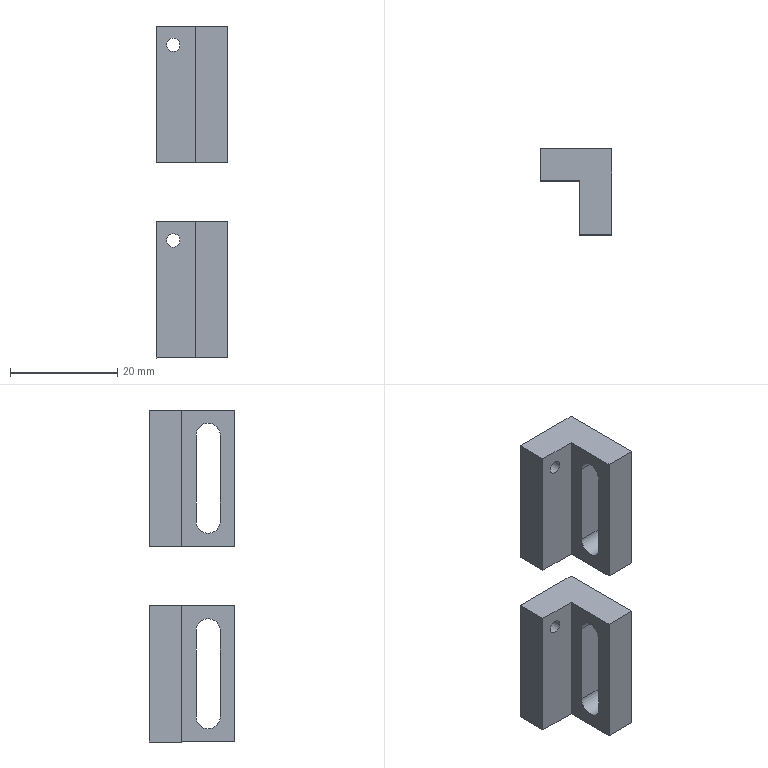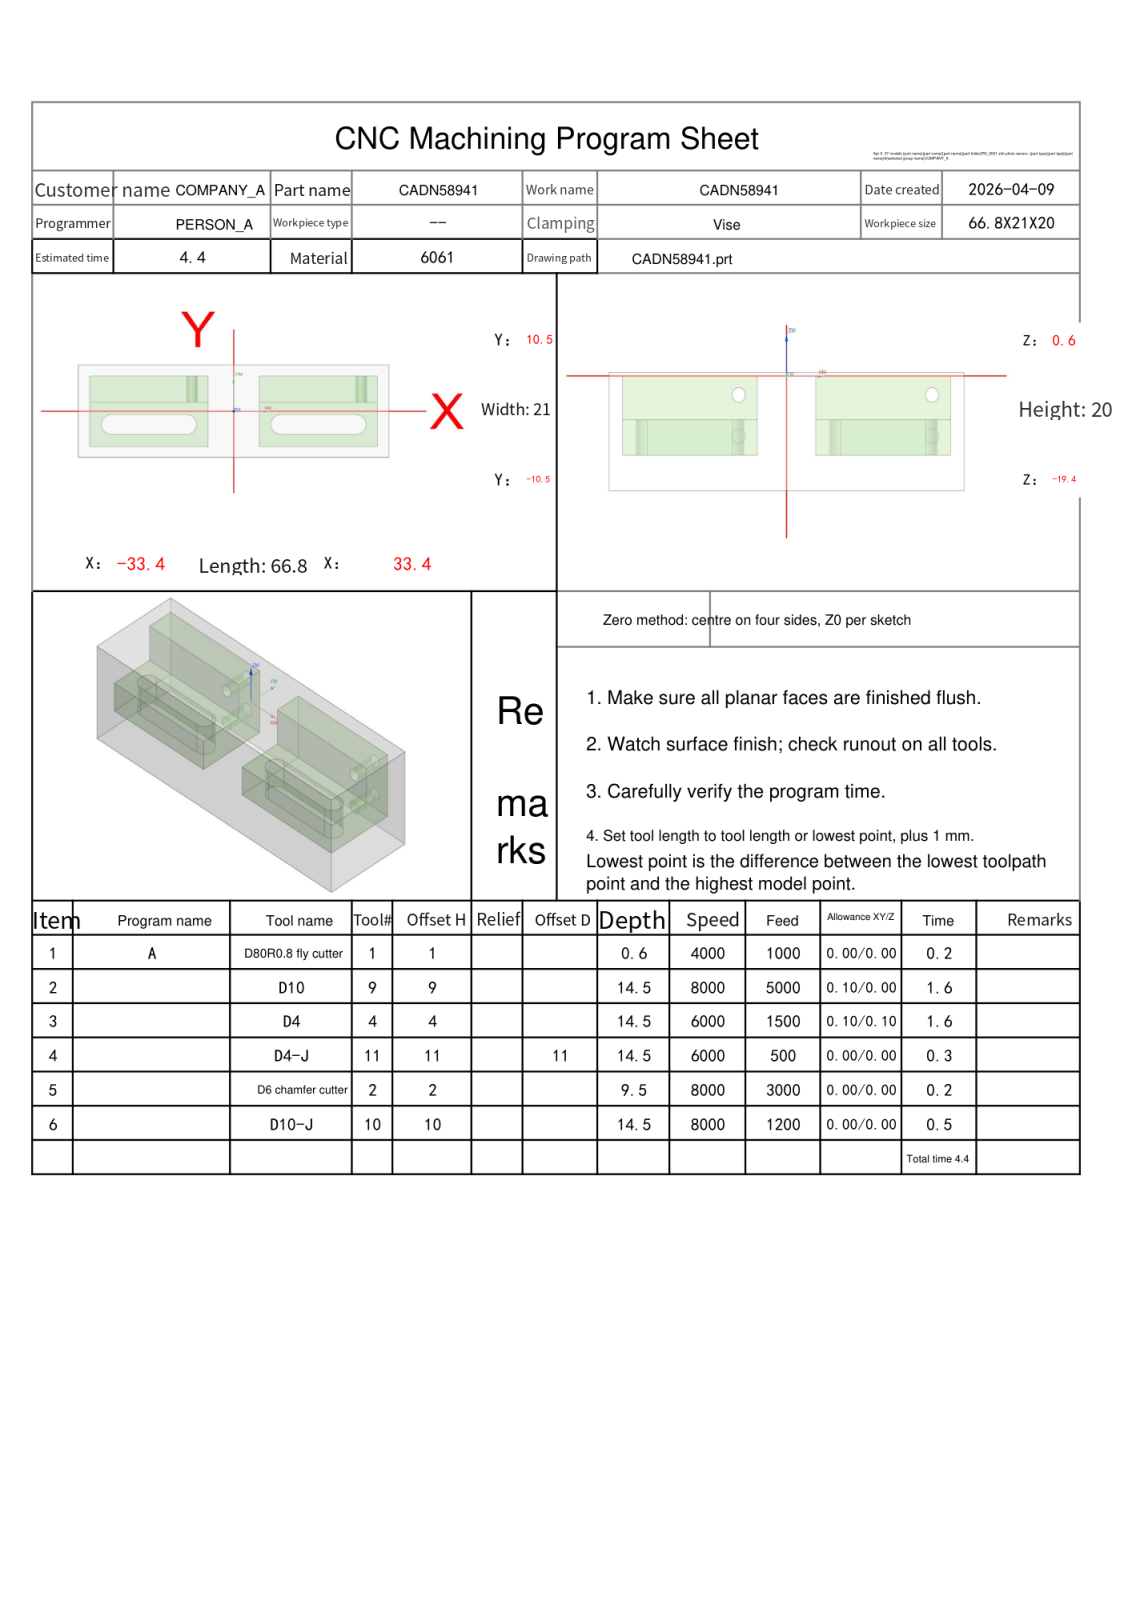NC program | NX | posted by the shop | part box 13.4 x 16 x 61.8 mm
Whole program:
%
O0001
(Machine time: 5.51 MIN)
(===Total Tool:6===)
(T1=D80R0.8 fly cutter D=80.  R=0.8  D-  H01 Z=-0.   )
(T9=D10     D=10.  R=0.   D-  H09 Z=-13.9 )
(T4=D4      D=4.   R=0.   D-  H04 Z=-13.9 )
(T11=D4-J   D=4.   R=0.   D11 H11 Z=-13.9 )
(T2=D6 chamfer cutter   D=6.   R=0.   D-  H02 Z=-8.9  )
(T10=D10-J  D=10.  R=0.   D10 H10 Z=-13.9 )
G80 G90 G17 G49 G40
G91 G28 Z0
M01
N1 T01 M06
(D80R0.8 fly cutter  D=80. R=0.8 H=01 ce=0.00 di=0.00)
G00 G90 G54 X-75.9 Y0.0 M03 S4000
G43 H01 Z20.
M08
Z2.
G01 Z0.0 F1000.
X-70.9
X70.9
X75.9
Z2.
G00 Z20.
G91 G28 Z0.0
M05
M09
G91 G28 Z0.0
M01
N2 T09 M06
(D10  D=10. R=0. H=09 ce=0.10 di=0.00)
G00 G90 G54 X18.2 Y-13.1 M03 S8000
G43 H09 Z20.
M08
Z.5
G01 X5.5 Z.412 F5000.
G02 X.4 Y-8. Z.356 I0.0 J5.1
G01 Y8. Z.244
G02 X5.5 Y13.1 Z.188 I5.1 J0.0
G01 X30.9 Z.012
G02 X36. Y8. Z-.044 I0.0 J-5.1
G01 Y-8. Z-.156
G02 X30.9 Y-13.1 Z-.212 I-5.1 J0.0
G01 X5.5 Z-.388
G02 X.4 Y-8. Z-.444 I0.0 J5.1
G01 Y8. Z-.556
G02 X5.5 Y13.1 Z-.612 I5.1 J0.0
G01 X30.9 Z-.788
G02 X36. Y8. Z-.844 I0.0 J-5.1
G01 Y-8. Z-.956
G02 X30.9 Y-13.1 Z-1.012 I-5.1 J0.0
G01 X5.5 Z-1.188
G02 X.4 Y-8. Z-1.244 I0.0 J5.1
G01 Y8. Z-1.356
G02 X5.5 Y13.1 Z-1.412 I5.1 J0.0
G01 X30.9 Z-1.588
G02 X36. Y8. Z-1.644 I0.0 J-5.1
G01 Y-8. Z-1.756
G02 X30.9 Y-13.1 Z-1.812 I-5.1 J0.0
G01 X5.5 Z-1.988
G02 X.4 Y-8. Z-2.044 I0.0 J5.1
G01 Y8. Z-2.156
G02 X5.5 Y13.1 Z-2.212 I5.1 J0.0
G01 X30.9 Z-2.388
G02 X36. Y8. Z-2.444 I0.0 J-5.1
G01 Y-8. Z-2.556
G02 X30.9 Y-13.1 Z-2.612 I-5.1 J0.0
G01 X5.5 Z-2.788
G02 X.4 Y-8. Z-2.844 I0.0 J5.1
G01 Y8. Z-2.956
G02 X5.5 Y13.1 Z-3.012 I5.1 J0.0
G01 X30.9 Z-3.188
G02 X36. Y8. Z-3.244 I0.0 J-5.1
G01 Y-8. Z-3.356
G02 X30.9 Y-13.1 Z-3.412 I-5.1 J0.0
G01 X5.5 Z-3.588
G02 X.4 Y-8. Z-3.644 I0.0 J5.1
G01 Y8. Z-3.756
G02 X5.5 Y13.1 Z-3.812 I5.1 J0.0
G01 X30.9 Z-3.988
G02 X36. Y8. Z-4.044 I0.0 J-5.1
G01 Y-8. Z-4.156
G02 X30.9 Y-13.1 Z-4.212 I-5.1 J0.0
G01 X5.5 Z-4.388
G02 X.4 Y-8. Z-4.444 I0.0 J5.1
G01 Y8. Z-4.556
G02 X5.5 Y13.1 Z-4.612 I5.1 J0.0
G01 X30.9 Z-4.788
G02 X36. Y8. Z-4.844 I0.0 J-5.1
G01 Y-8. Z-4.956
G02 X30.9 Y-13.1 Z-5.012 I-5.1 J0.0
G01 X5.5 Z-5.188
G02 X.4 Y-8. Z-5.244 I0.0 J5.1
G01 Y8. Z-5.356
G02 X5.5 Y13.1 Z-5.412 I5.1 J0.0
G01 X30.9 Z-5.588
G02 X36. Y8. Z-5.644 I0.0 J-5.1
G01 Y-8. Z-5.756
G02 X30.9 Y-13.1 Z-5.812 I-5.1 J0.0
G01 X5.5 Z-5.988
G02 X.4 Y-8. Z-6.044 I0.0 J5.1
G01 Y8. Z-6.156
G02 X5.5 Y13.1 Z-6.212 I5.1 J0.0
G01 X30.9 Z-6.388
G02 X36. Y8. Z-6.444 I0.0 J-5.1
G01 Y-8. Z-6.556
G02 X30.9 Y-13.1 Z-6.612 I-5.1 J0.0
G01 X5.5 Z-6.788
G02 X.4 Y-8. Z-6.844 I0.0 J5.1
G01 Y8. Z-6.956
G02 X5.5 Y13.1 Z-7.012 I5.1 J0.0
G01 X30.9 Z-7.188
G02 X36. Y8. Z-7.244 I0.0 J-5.1
G01 Y-8. Z-7.356
G02 X30.9 Y-13.1 Z-7.412 I-5.1 J0.0
G01 X5.5 Z-7.588
G02 X.4 Y-8. Z-7.644 I0.0 J5.1
G01 Y8. Z-7.756
G02 X5.5 Y13.1 Z-7.812 I5.1 J0.0
G01 X30.9 Z-7.988
G02 X36. Y8. Z-8.044 I0.0 J-5.1
G01 Y-8. Z-8.156
G02 X30.9 Y-13.1 Z-8.212 I-5.1 J0.0
G01 X5.5 Z-8.388
G02 X.4 Y-8. Z-8.444 I0.0 J5.1
G01 Y8. Z-8.556
G02 X5.5 Y13.1 Z-8.612 I5.1 J0.0
G01 X30.9 Z-8.788
G02 X36. Y8. Z-8.844 I0.0 J-5.1
G01 Y-8. Z-8.956
G02 X30.9 Y-13.1 Z-9.012 I-5.1 J0.0
G01 X5.5 Z-9.188
G02 X.4 Y-8. Z-9.244 I0.0 J5.1
G01 Y8. Z-9.356
G02 X5.5 Y13.1 Z-9.412 I5.1 J0.0
G01 X30.9 Z-9.588
G02 X36. Y8. Z-9.644 I0.0 J-5.1
G01 Y-8. Z-9.756
G02 X30.9 Y-13.1 Z-9.812 I-5.1 J0.0
G01 X5.5 Z-9.988
G02 X.4 Y-8. Z-10.044 I0.0 J5.1
G01 Y8. Z-10.156
G02 X5.5 Y13.1 Z-10.212 I5.1 J0.0
G01 X30.9 Z-10.388
G02 X36. Y8. Z-10.444 I0.0 J-5.1
G01 Y-8. Z-10.556
G02 X30.9 Y-13.1 Z-10.612 I-5.1 J0.0
G01 X5.5 Z-10.788
G02 X.4 Y-8. Z-10.844 I0.0 J5.1
G01 Y8. Z-10.956
G02 X5.5 Y13.1 Z-11.012 I5.1 J0.0
G01 X30.9 Z-11.188
G02 X36. Y8. Z-11.244 I0.0 J-5.1
G01 Y-8. Z-11.356
G02 X30.9 Y-13.1 Z-11.412 I-5.1 J0.0
G01 X5.5 Z-11.588
G02 X.4 Y-8. Z-11.644 I0.0 J5.1
G01 Y8. Z-11.756
G02 X5.5 Y13.1 Z-11.812 I5.1 J0.0
G01 X30.9 Z-11.988
G02 X36. Y8. Z-12.044 I0.0 J-5.1
G01 Y-8. Z-12.156
G02 X30.9 Y-13.1 Z-12.212 I-5.1 J0.0
G01 X5.5 Z-12.388
G02 X.4 Y-8. Z-12.444 I0.0 J5.1
G01 Y8. Z-12.556
G02 X5.5 Y13.1 Z-12.612 I5.1 J0.0
G01 X30.9 Z-12.788
G02 X36. Y8. Z-12.844 I0.0 J-5.1
G01 Y-8. Z-12.956
G02 X30.9 Y-13.1 Z-13.012 I-5.1 J0.0
G01 X5.5 Z-13.188
G02 X.4 Y-8. Z-13.244 I0.0 J5.1
G01 Y8. Z-13.356
G02 X5.5 Y13.1 Z-13.412 I5.1 J0.0
G01 X30.9 Z-13.588
G02 X36. Y8. Z-13.644 I0.0 J-5.1
G01 Y-8. Z-13.756
G02 X30.9 Y-13.1 Z-13.812 I-5.1 J0.0
G01 X18.2 Z-13.9
X5.5
G02 X.4 Y-8. I0.0 J5.1
G01 Y8.
G02 X5.5 Y13.1 I5.1 J0.0
G01 X30.9
G02 X36. Y8. I0.0 J-5.1
G01 Y-8.
G02 X30.9 Y-13.1 I-5.1 J0.0
G01 X18.2
X17.7
Z-12.9
G00 Z20.
X-18.2
Z.5
G01 X-30.9 Z.412
G02 X-36. Y-8. Z.356 I0.0 J5.1
G01 Y8. Z.244
G02 X-30.9 Y13.1 Z.188 I5.1 J0.0
G01 X-5.5 Z.012
G02 X-.4 Y8. Z-.044 I0.0 J-5.1
G01 Y-8. Z-.156
G02 X-5.5 Y-13.1 Z-.212 I-5.1 J0.0
G01 X-30.9 Z-.388
G02 X-36. Y-8. Z-.444 I0.0 J5.1
G01 Y8. Z-.556
G02 X-30.9 Y13.1 Z-.612 I5.1 J0.0
G01 X-5.5 Z-.788
G02 X-.4 Y8. Z-.844 I0.0 J-5.1
G01 Y-8. Z-.956
G02 X-5.5 Y-13.1 Z-1.012 I-5.1 J0.0
G01 X-30.9 Z-1.188
G02 X-36. Y-8. Z-1.244 I0.0 J5.1
G01 Y8. Z-1.356
G02 X-30.9 Y13.1 Z-1.412 I5.1 J0.0
G01 X-5.5 Z-1.588
G02 X-.4 Y8. Z-1.644 I0.0 J-5.1
G01 Y-8. Z-1.756
G02 X-5.5 Y-13.1 Z-1.812 I-5.1 J0.0
G01 X-30.9 Z-1.988
G02 X-36. Y-8. Z-2.044 I0.0 J5.1
G01 Y8. Z-2.156
G02 X-30.9 Y13.1 Z-2.212 I5.1 J0.0
G01 X-5.5 Z-2.388
G02 X-.4 Y8. Z-2.444 I0.0 J-5.1
G01 Y-8. Z-2.556
G02 X-5.5 Y-13.1 Z-2.612 I-5.1 J0.0
G01 X-30.9 Z-2.788
G02 X-36. Y-8. Z-2.844 I0.0 J5.1
G01 Y8. Z-2.956
G02 X-30.9 Y13.1 Z-3.012 I5.1 J0.0
G01 X-5.5 Z-3.188
G02 X-.4 Y8. Z-3.244 I0.0 J-5.1
G01 Y-8. Z-3.356
G02 X-5.5 Y-13.1 Z-3.412 I-5.1 J0.0
G01 X-30.9 Z-3.588
G02 X-36. Y-8. Z-3.644 I0.0 J5.1
G01 Y8. Z-3.756
G02 X-30.9 Y13.1 Z-3.812 I5.1 J0.0
G01 X-5.5 Z-3.988
G02 X-.4 Y8. Z-4.044 I0.0 J-5.1
G01 Y-8. Z-4.156
G02 X-5.5 Y-13.1 Z-4.212 I-5.1 J0.0
G01 X-30.9 Z-4.388
G02 X-36. Y-8. Z-4.444 I0.0 J5.1
G01 Y8. Z-4.556
G02 X-30.9 Y13.1 Z-4.612 I5.1 J0.0
G01 X-5.5 Z-4.788
G02 X-.4 Y8. Z-4.844 I0.0 J-5.1
G01 Y-8. Z-4.956
G02 X-5.5 Y-13.1 Z-5.012 I-5.1 J0.0
G01 X-30.9 Z-5.188
G02 X-36. Y-8. Z-5.244 I0.0 J5.1
G01 Y8. Z-5.356
G02 X-30.9 Y13.1 Z-5.412 I5.1 J0.0
G01 X-5.5 Z-5.588
G02 X-.4 Y8. Z-5.644 I0.0 J-5.1
G01 Y-8. Z-5.756
G02 X-5.5 Y-13.1 Z-5.812 I-5.1 J0.0
G01 X-30.9 Z-5.988
G02 X-36. Y-8. Z-6.044 I0.0 J5.1
G01 Y8. Z-6.156
G02 X-30.9 Y13.1 Z-6.212 I5.1 J0.0
G01 X-5.5 Z-6.388
G02 X-.4 Y8. Z-6.444 I0.0 J-5.1
G01 Y-8. Z-6.556
G02 X-5.5 Y-13.1 Z-6.612 I-5.1 J0.0
G01 X-30.9 Z-6.788
G02 X-36. Y-8. Z-6.844 I0.0 J5.1
G01 Y8. Z-6.956
G02 X-30.9 Y13.1 Z-7.012 I5.1 J0.0
G01 X-5.5 Z-7.188
G02 X-.4 Y8. Z-7.244 I0.0 J-5.1
G01 Y-8. Z-7.356
G02 X-5.5 Y-13.1 Z-7.412 I-5.1 J0.0
G01 X-30.9 Z-7.588
G02 X-36. Y-8. Z-7.644 I0.0 J5.1
G01 Y8. Z-7.756
G02 X-30.9 Y13.1 Z-7.812 I5.1 J0.0
G01 X-5.5 Z-7.988
G02 X-.4 Y8. Z-8.044 I0.0 J-5.1
G01 Y-8. Z-8.156
G02 X-5.5 Y-13.1 Z-8.212 I-5.1 J0.0
G01 X-30.9 Z-8.388
G02 X-36. Y-8. Z-8.444 I0.0 J5.1
G01 Y8. Z-8.556
G02 X-30.9 Y13.1 Z-8.612 I5.1 J0.0
G01 X-5.5 Z-8.788
G02 X-.4 Y8. Z-8.844 I0.0 J-5.1
G01 Y-8. Z-8.956
G02 X-5.5 Y-13.1 Z-9.012 I-5.1 J0.0
G01 X-30.9 Z-9.188
G02 X-36. Y-8. Z-9.244 I0.0 J5.1
G01 Y8. Z-9.356
G02 X-30.9 Y13.1 Z-9.412 I5.1 J0.0
G01 X-5.5 Z-9.588
G02 X-.4 Y8. Z-9.644 I0.0 J-5.1
G01 Y-8. Z-9.756
G02 X-5.5 Y-13.1 Z-9.812 I-5.1 J0.0
G01 X-30.9 Z-9.988
G02 X-36. Y-8. Z-10.044 I0.0 J5.1
G01 Y8. Z-10.156
G02 X-30.9 Y13.1 Z-10.212 I5.1 J0.0
G01 X-5.5 Z-10.388
G02 X-.4 Y8. Z-10.444 I0.0 J-5.1
G01 Y-8. Z-10.556
G02 X-5.5 Y-13.1 Z-10.612 I-5.1 J0.0
G01 X-30.9 Z-10.788
G02 X-36. Y-8. Z-10.844 I0.0 J5.1
G01 Y8. Z-10.956
G02 X-30.9 Y13.1 Z-11.012 I5.1 J0.0
G01 X-5.5 Z-11.188
G02 X-.4 Y8. Z-11.244 I0.0 J-5.1
G01 Y-8. Z-11.356
G02 X-5.5 Y-13.1 Z-11.412 I-5.1 J0.0
G01 X-30.9 Z-11.588
G02 X-36. Y-8. Z-11.644 I0.0 J5.1
G01 Y8. Z-11.756
G02 X-30.9 Y13.1 Z-11.812 I5.1 J0.0
G01 X-5.5 Z-11.988
G02 X-.4 Y8. Z-12.044 I0.0 J-5.1
G01 Y-8. Z-12.156
G02 X-5.5 Y-13.1 Z-12.212 I-5.1 J0.0
G01 X-30.9 Z-12.388
G02 X-36. Y-8. Z-12.444 I0.0 J5.1
G01 Y8. Z-12.556
G02 X-30.9 Y13.1 Z-12.612 I5.1 J0.0
G01 X-5.5 Z-12.788
G02 X-.4 Y8. Z-12.844 I0.0 J-5.1
G01 Y-8. Z-12.956
G02 X-5.5 Y-13.1 Z-13.012 I-5.1 J0.0
G01 X-30.9 Z-13.188
G02 X-36. Y-8. Z-13.244 I0.0 J5.1
G01 Y8. Z-13.356
G02 X-30.9 Y13.1 Z-13.412 I5.1 J0.0
G01 X-5.5 Z-13.588
G02 X-.4 Y8. Z-13.644 I0.0 J-5.1
G01 Y-8. Z-13.756
G02 X-5.5 Y-13.1 Z-13.812 I-5.1 J0.0
G01 X-18.2 Z-13.9
X-30.9
G02 X-36. Y-8. I0.0 J5.1
G01 Y8.
G02 X-30.9 Y13.1 I5.1 J0.0
G01 X-5.5
G02 X-.4 Y8. I0.0 J-5.1
G01 Y-8.
G02 X-5.5 Y-13.1 I-5.1 J0.0
G01 X-18.2
X-18.7
Z-12.9
G00 Z20.
G00 G90 X18.2 Y-16. M03 S8000
Z20.
Z.013
G01 Z-.487 F3500.
Y-9.
X31.9
Y-3.1
X4.5
Y-9.
X18.2
X18.7
Z.013
G00 Z.5
X18.2 Y-16.
Z-.473
G01 Z-.973
Y-9.
X31.9
Y-3.1
X4.5
Y-9.
X18.2
X18.7
Z-.473
G00 Z.013
X18.2 Y-16.
Z-.96
G01 Z-1.46
Y-9.
X31.9
Y-3.1
X4.5
Y-9.
X18.2
X18.7
Z-.96
G00 Z-.473
X18.2 Y-16.
Z-1.447
G01 Z-1.947
Y-9.
X31.9
Y-3.1
X4.5
Y-9.
X18.2
X18.7
Z-1.447
G00 Z-.96
X18.2 Y-16.
Z-1.933
G01 Z-2.433
Y-9.
X31.9
Y-3.1
X4.5
Y-9.
X18.2
X18.7
Z-1.933
G00 Z-1.447
X18.2 Y-16.
Z-2.42
G01 Z-2.92
Y-9.
X31.9
Y-3.1
X4.5
Y-9.
X18.2
X18.7
Z-2.42
G00 Z-1.933
X18.2 Y-16.
Z-2.907
G01 Z-3.407
Y-9.
X31.9
Y-3.1
X4.5
Y-9.
X18.2
X18.7
Z-2.907
G00 Z-2.42
X18.2 Y-16.
Z-3.393
G01 Z-3.893
Y-9.
X31.9
Y-3.1
X4.5
Y-9.
X18.2
X18.7
Z-3.393
G00 Z-2.907
X18.2 Y-16.
Z-3.88
G01 Z-4.38
Y-9.
X31.9
Y-3.1
X4.5
Y-9.
X18.2
X18.7
Z-3.88
G00 Z-3.393
X18.2 Y-16.
Z-4.367
G01 Z-4.867
Y-9.
X31.9
Y-3.1
X4.5
Y-9.
X18.2
X18.7
Z-4.367
G00 Z-3.88
X18.2 Y-16.
Z-4.853
G01 Z-5.353
Y-9.
X31.9
Y-3.1
X4.5
Y-9.
X18.2
X18.7
Z-4.853
G00 Z-4.367
X18.2 Y-16.
Z-5.34
G01 Z-5.84
Y-9.
X31.9
Y-3.1
X4.5
Y-9.
X18.2
X18.7
Z-5.34
G00 Z-4.853
X18.2 Y-16.
Z-5.827
G01 Z-6.327
Y-9.
X31.9
Y-3.1
X4.5
Y-9.
X18.2
X18.7
Z-5.827
G00 Z-5.34
X18.2 Y-16.
Z-6.313
G01 Z-6.813
Y-9.
X31.9
Y-3.1
X4.5
Y-9.
X18.2
X18.7
Z-6.313
G00 Z-5.827
X18.2 Y-16.
Z-6.8
G01 Z-7.3
Y-9.
X31.9
Y-3.1
X4.5
Y-9.
X18.2
X18.7
Z-6.8
G00 Z20.
X-18.2 Y-16.
Z.013
G01 Z-.487
Y-9.
X-4.5
Y-3.1
X-31.9
Y-9.
X-18.2
X-17.7
Z.013
G00 Z.5
X-18.2 Y-16.
Z-.473
G01 Z-.973
Y-9.
X-4.5
Y-3.1
X-31.9
Y-9.
X-18.2
X-17.7
Z-.473
G00 Z.013
X-18.2 Y-16.
Z-.96
G01 Z-1.46
Y-9.
X-4.5
Y-3.1
X-31.9
Y-9.
X-18.2
X-17.7
Z-.96
G00 Z-.473
X-18.2 Y-16.
Z-1.447
G01 Z-1.947
Y-9.
X-4.5
Y-3.1
X-31.9
Y-9.
X-18.2
X-17.7
Z-1.447
G00 Z-.96
X-18.2 Y-16.
Z-1.933
G01 Z-2.433
Y-9.
X-4.5
Y-3.1
X-31.9
Y-9.
X-18.2
X-17.7
Z-1.933
G00 Z-1.447
X-18.2 Y-16.
Z-2.42
G01 Z-2.92
Y-9.
X-4.5
Y-3.1
X-31.9
Y-9.
X-18.2
X-17.7
Z-2.42
G00 Z-1.933
X-18.2 Y-16.
Z-2.907
G01 Z-3.407
Y-9.
X-4.5
Y-3.1
X-31.9
Y-9.
X-18.2
X-17.7
Z-2.907
G00 Z-2.42
X-18.2 Y-16.
Z-3.393
G01 Z-3.893
Y-9.
X-4.5
Y-3.1
X-31.9
Y-9.
X-18.2
X-17.7
Z-3.393
G00 Z-2.907
X-18.2 Y-16.
Z-3.88
G01 Z-4.38
Y-9.
X-4.5
Y-3.1
X-31.9
Y-9.
X-18.2
X-17.7
Z-3.88
G00 Z-3.393
X-18.2 Y-16.
Z-4.367
G01 Z-4.867
Y-9.
X-4.5
Y-3.1
X-31.9
Y-9.
X-18.2
X-17.7
Z-4.367
G00 Z-3.88
X-18.2 Y-16.
Z-4.853
G01 Z-5.353
Y-9.
X-4.5
Y-3.1
X-31.9
Y-9.
X-18.2
X-17.7
Z-4.853
G00 Z-4.367
X-18.2 Y-16.
Z-5.34
G01 Z-5.84
Y-9.
X-4.5
Y-3.1
X-31.9
Y-9.
X-18.2
X-17.7
Z-5.34
G00 Z-4.853
X-18.2 Y-16.
Z-5.827
G01 Z-6.327
Y-9.
X-4.5
Y-3.1
X-31.9
Y-9.
X-18.2
X-17.7
Z-5.827
G00 Z-5.34
X-18.2 Y-16.
Z-6.313
G01 Z-6.813
Y-9.
X-4.5
Y-3.1
X-31.9
Y-9.
X-18.2
X-17.7
Z-6.313
G00 Z-5.827
X-18.2 Y-16.
Z-6.8
G01 Z-7.3
Y-9.
X-4.5
Y-3.1
X-31.9
Y-9.
X-18.2
X-17.7
Z-6.8
G00 Z20.
G91 G28 Z0.0
M05
M09
G91 G28 Z0.0
M01
N3 T04 M06
(D4  D=4. R=0. H=04 ce=0.10 di=0.10)
G00 G90 G54 X-18.2 Y-3.15 M03 S6000
G43 H04 Z20.
M08
Z-6.9
G01 X-10.2 Z-6.947 F1500.
G03 X-10.05 Y-3. Z-6.949 I0.0 J.15
X-10.2 Y-2.85 Z-6.95 I-.15 J0.0
G01 X-26.2 Z-7.044
G03 X-26.35 Y-3. Z-7.046 I0.0 J-.15
X-26.2 Y-3.15 Z-7.047 I.15 J0.0
G01 X-10.2 Z-7.142
G03 X-10.05 Y-3. Z-7.143 I0.0 J.15
X-10.2 Y-2.85 Z-7.144 I-.15 J0.0
G01 X-26.2 Z-7.239
G03 X-26.35 Y-3. Z-7.24 I0.0 J-.15
X-26.2 Y-3.15 Z-7.242 I.15 J0.0
G01 X-10.2 Z-7.336
G03 X-10.05 Y-3. Z-7.338 I0.0 J.15
X-10.2 Y-2.85 Z-7.339 I-.15 J0.0
G01 X-26.2 Z-7.433
G03 X-26.35 Y-3. Z-7.435 I0.0 J-.15
X-26.2 Y-3.15 Z-7.436 I.15 J0.0
G01 X-10.2 Z-7.531
G03 X-10.05 Y-3. Z-7.532 I0.0 J.15
X-10.2 Y-2.85 Z-7.533 I-.15 J0.0
G01 X-26.2 Z-7.628
G03 X-26.35 Y-3. Z-7.629 I0.0 J-.15
X-26.2 Y-3.15 Z-7.631 I.15 J0.0
G01 X-10.2 Z-7.725
G03 X-10.05 Y-3. Z-7.726 I0.0 J.15
X-10.2 Y-2.85 Z-7.728 I-.15 J0.0
G01 X-26.2 Z-7.822
G03 X-26.35 Y-3. Z-7.824 I0.0 J-.15
X-26.2 Y-3.15 Z-7.825 I.15 J0.0
G01 X-10.2 Z-7.919
G03 X-10.05 Y-3. Z-7.921 I0.0 J.15
X-10.2 Y-2.85 Z-7.922 I-.15 J0.0
G01 X-26.2 Z-8.017
G03 X-26.35 Y-3. Z-8.018 I0.0 J-.15
X-26.2 Y-3.15 Z-8.019 I.15 J0.0
G01 X-10.2 Z-8.114
G03 X-10.05 Y-3. Z-8.115 I0.0 J.15
X-10.2 Y-2.85 Z-8.117 I-.15 J0.0
G01 X-26.2 Z-8.211
G03 X-26.35 Y-3. Z-8.213 I0.0 J-.15
X-26.2 Y-3.15 Z-8.214 I.15 J0.0
G01 X-10.2 Z-8.308
G03 X-10.05 Y-3. Z-8.31 I0.0 J.15
X-10.2 Y-2.85 Z-8.311 I-.15 J0.0
G01 X-26.2 Z-8.406
G03 X-26.35 Y-3. Z-8.407 I0.0 J-.15
X-26.2 Y-3.15 Z-8.408 I.15 J0.0
G01 X-10.2 Z-8.503
G03 X-10.05 Y-3. Z-8.504 I0.0 J.15
X-10.2 Y-2.85 Z-8.506 I-.15 J0.0
G01 X-26.2 Z-8.6
G03 X-26.35 Y-3. Z-8.601 I0.0 J-.15
X-26.2 Y-3.15 Z-8.603 I.15 J0.0
G01 X-10.2 Z-8.697
G03 X-10.05 Y-3. Z-8.699 I0.0 J.15
X-10.2 Y-2.85 Z-8.7 I-.15 J0.0
G01 X-26.2 Z-8.794
G03 X-26.35 Y-3. Z-8.796 I0.0 J-.15
X-26.2 Y-3.15 Z-8.797 I.15 J0.0
G01 X-10.2 Z-8.892
G03 X-10.05 Y-3. Z-8.893 I0.0 J.15
X-10.2 Y-2.85 Z-8.894 I-.15 J0.0
G01 X-26.2 Z-8.989
G03 X-26.35 Y-3. Z-8.99 I0.0 J-.15
X-26.2 Y-3.15 Z-8.992 I.15 J0.0
G01 X-10.2 Z-9.086
G03 X-10.05 Y-3. Z-9.088 I0.0 J.15
X-10.2 Y-2.85 Z-9.089 I-.15 J0.0
G01 X-26.2 Z-9.183
G03 X-26.35 Y-3. Z-9.185 I0.0 J-.15
X-26.2 Y-3.15 Z-9.186 I.15 J0.0
G01 X-10.2 Z-9.281
G03 X-10.05 Y-3. Z-9.282 I0.0 J.15
X-10.2 Y-2.85 Z-9.283 I-.15 J0.0
G01 X-26.2 Z-9.378
G03 X-26.35 Y-3. Z-9.379 I0.0 J-.15
X-26.2 Y-3.15 Z-9.381 I.15 J0.0
G01 X-10.2 Z-9.475
G03 X-10.05 Y-3. Z-9.476 I0.0 J.15
X-10.2 Y-2.85 Z-9.478 I-.15 J0.0
G01 X-26.2 Z-9.572
G03 X-26.35 Y-3. Z-9.574 I0.0 J-.15
X-26.2 Y-3.15 Z-9.575 I.15 J0.0
G01 X-10.2 Z-9.669
G03 X-10.05 Y-3. Z-9.671 I0.0 J.15
X-10.2 Y-2.85 Z-9.672 I-.15 J0.0
G01 X-26.2 Z-9.767
G03 X-26.35 Y-3. Z-9.768 I0.0 J-.15
X-26.2 Y-3.15 Z-9.769 I.15 J0.0
G01 X-10.2 Z-9.864
G03 X-10.05 Y-3. Z-9.865 I0.0 J.15
X-10.2 Y-2.85 Z-9.867 I-.15 J0.0
G01 X-26.2 Z-9.961
G03 X-26.35 Y-3. Z-9.963 I0.0 J-.15
X-26.2 Y-3.15 Z-9.964 I.15 J0.0
G01 X-10.2 Z-10.058
G03 X-10.05 Y-3. Z-10.06 I0.0 J.15
X-10.2 Y-2.85 Z-10.061 I-.15 J0.0
G01 X-26.2 Z-10.156
G03 X-26.35 Y-3. Z-10.157 I0.0 J-.15
X-26.2 Y-3.15 Z-10.158 I.15 J0.0
G01 X-10.2 Z-10.253
G03 X-10.05 Y-3. Z-10.254 I0.0 J.15
X-10.2 Y-2.85 Z-10.256 I-.15 J0.0
G01 X-26.2 Z-10.35
G03 X-26.35 Y-3. Z-10.351 I0.0 J-.15
X-26.2 Y-3.15 Z-10.353 I.15 J0.0
G01 X-10.2 Z-10.447
G03 X-10.05 Y-3. Z-10.449 I0.0 J.15
X-10.2 Y-2.85 Z-10.45 I-.15 J0.0
G01 X-26.2 Z-10.544
G03 X-26.35 Y-3. Z-10.546 I0.0 J-.15
X-26.2 Y-3.15 Z-10.547 I.15 J0.0
G01 X-10.2 Z-10.642
G03 X-10.05 Y-3. Z-10.643 I0.0 J.15
X-10.2 Y-2.85 Z-10.644 I-.15 J0.0
G01 X-26.2 Z-10.739
G03 X-26.35 Y-3. Z-10.74 I0.0 J-.15
X-26.2 Y-3.15 Z-10.742 I.15 J0.0
G01 X-10.2 Z-10.836
G03 X-10.05 Y-3. Z-10.838 I0.0 J.15
X-10.2 Y-2.85 Z-10.839 I-.15 J0.0
G01 X-26.2 Z-10.933
G03 X-26.35 Y-3. Z-10.935 I0.0 J-.15
X-26.2 Y-3.15 Z-10.936 I.15 J0.0
G01 X-10.2 Z-11.031
G03 X-10.05 Y-3. Z-11.032 I0.0 J.15
X-10.2 Y-2.85 Z-11.033 I-.15 J0.0
G01 X-26.2 Z-11.128
G03 X-26.35 Y-3. Z-11.129 I0.0 J-.15
X-26.2 Y-3.15 Z-11.131 I.15 J0.0
G01 X-10.2 Z-11.225
G03 X-10.05 Y-3. Z-11.226 I0.0 J.15
X-10.2 Y-2.85 Z-11.228 I-.15 J0.0
G01 X-26.2 Z-11.322
G03 X-26.35 Y-3. Z-11.324 I0.0 J-.15
X-26.2 Y-3.15 Z-11.325 I.15 J0.0
G01 X-10.2 Z-11.419
G03 X-10.05 Y-3. Z-11.421 I0.0 J.15
X-10.2 Y-2.85 Z-11.422 I-.15 J0.0
G01 X-26.2 Z-11.517
G03 X-26.35 Y-3. Z-11.518 I0.0 J-.15
X-26.2 Y-3.15 Z-11.519 I.15 J0.0
G01 X-10.2 Z-11.614
G03 X-10.05 Y-3. Z-11.615 I0.0 J.15
X-10.2 Y-2.85 Z-11.617 I-.15 J0.0
G01 X-26.2 Z-11.711
G03 X-26.35 Y-3. Z-11.713 I0.0 J-.15
X-26.2 Y-3.15 Z-11.714 I.15 J0.0
G01 X-10.2 Z-11.808
G03 X-10.05 Y-3. Z-11.81 I0.0 J.15
X-10.2 Y-2.85 Z-11.811 I-.15 J0.0
G01 X-26.2 Z-11.906
G03 X-26.35 Y-3. Z-11.907 I0.0 J-.15
X-26.2 Y-3.15 Z-11.908 I.15 J0.0
G01 X-10.2 Z-12.003
G03 X-10.05 Y-3. Z-12.004 I0.0 J.15
X-10.2 Y-2.85 Z-12.006 I-.15 J0.0
G01 X-26.2 Z-12.1
G03 X-26.35 Y-3. Z-12.101 I0.0 J-.15
X-26.2 Y-3.15 Z-12.103 I.15 J0.0
G01 X-10.2 Z-12.197
G03 X-10.05 Y-3. Z-12.199 I0.0 J.15
X-10.2 Y-2.85 Z-12.2 I-.15 J0.0
G01 X-26.2 Z-12.294
G03 X-26.35 Y-3. Z-12.296 I0.0 J-.15
X-26.2 Y-3.15 Z-12.297 I.15 J0.0
G01 X-10.2 Z-12.392
G03 X-10.05 Y-3. Z-12.393 I0.0 J.15
X-10.2 Y-2.85 Z-12.394 I-.15 J0.0
G01 X-26.2 Z-12.489
G03 X-26.35 Y-3. Z-12.49 I0.0 J-.15
X-26.2 Y-3.15 Z-12.492 I.15 J0.0
G01 X-10.2 Z-12.586
G03 X-10.05 Y-3. Z-12.588 I0.0 J.15
X-10.2 Y-2.85 Z-12.589 I-.15 J0.0
G01 X-26.2 Z-12.683
G03 X-26.35 Y-3. Z-12.685 I0.0 J-.15
X-26.2 Y-3.15 Z-12.686 I.15 J0.0
G01 X-10.2 Z-12.781
G03 X-10.05 Y-3. Z-12.782 I0.0 J.15
X-10.2 Y-2.85 Z-12.783 I-.15 J0.0
G01 X-26.2 Z-12.878
G03 X-26.35 Y-3. Z-12.879 I0.0 J-.15
X-26.2 Y-3.15 Z-12.881 I.15 J0.0
G01 X-10.2 Z-12.975
G03 X-10.05 Y-3. Z-12.976 I0.0 J.15
X-10.2 Y-2.85 Z-12.978 I-.15 J0.0
G01 X-26.2 Z-13.072
G03 X-26.35 Y-3. Z-13.074 I0.0 J-.15
X-26.2 Y-3.15 Z-13.075 I.15 J0.0
G01 X-10.2 Z-13.169
G03 X-10.05 Y-3. Z-13.171 I0.0 J.15
X-10.2 Y-2.85 Z-13.172 I-.15 J0.0
G01 X-26.2 Z-13.267
G03 X-26.35 Y-3. Z-13.268 I0.0 J-.15
X-26.2 Y-3.15 Z-13.269 I.15 J0.0
G01 X-10.2 Z-13.364
G03 X-10.05 Y-3. Z-13.365 I0.0 J.15
X-10.2 Y-2.85 Z-13.367 I-.15 J0.0
G01 X-26.2 Z-13.461
G03 X-26.35 Y-3. Z-13.463 I0.0 J-.15
X-26.2 Y-3.15 Z-13.464 I.15 J0.0
G01 X-10.2 Z-13.558
G03 X-10.05 Y-3. Z-13.56 I0.0 J.15
X-10.2 Y-2.85 Z-13.561 I-.15 J0.0
G01 X-26.2 Z-13.656
G03 X-26.35 Y-3. Z-13.657 I0.0 J-.15
X-26.2 Y-3.15 Z-13.658 I.15 J0.0
G01 X-10.2 Z-13.753
G03 X-10.05 Y-3. Z-13.754 I0.0 J.15
X-10.2 Y-2.85 Z-13.756 I-.15 J0.0
G01 X-26.2 Z-13.85
G03 X-26.35 Y-3. Z-13.851 I0.0 J-.15
X-26.2 Y-3.15 Z-13.853 I.15 J0.0
G01 X-18.2 Z-13.9
X-10.2
G03 X-10.05 Y-3. I0.0 J.15
X-10.2 Y-2.85 I-.15 J0.0
G01 X-26.2
G03 X-26.35 Y-3. I0.0 J-.15
X-26.2 Y-3.15 I.15 J0.0
G01 X-18.2
X-17.7
Z-12.9
G00 Z20.
X18.2
Z-6.9
G01 X26.2 Z-6.947
G03 X26.35 Y-3. Z-6.949 I0.0 J.15
X26.2 Y-2.85 Z-6.95 I-.15 J0.0
G01 X10.2 Z-7.044
G03 X10.05 Y-3. Z-7.046 I0.0 J-.15
X10.2 Y-3.15 Z-7.047 I.15 J0.0
G01 X26.2 Z-7.142
G03 X26.35 Y-3. Z-7.143 I0.0 J.15
X26.2 Y-2.85 Z-7.144 I-.15 J0.0
G01 X10.2 Z-7.239
G03 X10.05 Y-3. Z-7.24 I0.0 J-.15
X10.2 Y-3.15 Z-7.242 I.15 J0.0
G01 X26.2 Z-7.336
G03 X26.35 Y-3. Z-7.338 I0.0 J.15
X26.2 Y-2.85 Z-7.339 I-.15 J0.0
G01 X10.2 Z-7.433
G03 X10.05 Y-3. Z-7.435 I0.0 J-.15
X10.2 Y-3.15 Z-7.436 I.15 J0.0
G01 X26.2 Z-7.531
G03 X26.35 Y-3. Z-7.532 I0.0 J.15
X26.2 Y-2.85 Z-7.533 I-.15 J0.0
G01 X10.2 Z-7.628
G03 X10.05 Y-3. Z-7.629 I0.0 J-.15
X10.2 Y-3.15 Z-7.631 I.15 J0.0
G01 X26.2 Z-7.725
G03 X26.35 Y-3. Z-7.726 I0.0 J.15
X26.2 Y-2.85 Z-7.728 I-.15 J0.0
G01 X10.2 Z-7.822
G03 X10.05 Y-3. Z-7.824 I0.0 J-.15
X10.2 Y-3.15 Z-7.825 I.15 J0.0
G01 X26.2 Z-7.919
G03 X26.35 Y-3. Z-7.921 I0.0 J.15
X26.2 Y-2.85 Z-7.922 I-.15 J0.0
G01 X10.2 Z-8.017
G03 X10.05 Y-3. Z-8.018 I0.0 J-.15
X10.2 Y-3.15 Z-8.019 I.15 J0.0
G01 X26.2 Z-8.114
G03 X26.35 Y-3. Z-8.115 I0.0 J.15
X26.2 Y-2.85 Z-8.117 I-.15 J0.0
G01 X10.2 Z-8.211
G03 X10.05 Y-3. Z-8.213 I0.0 J-.15
X10.2 Y-3.15 Z-8.214 I.15 J0.0
G01 X26.2 Z-8.308
G03 X26.35 Y-3. Z-8.31 I0.0 J.15
X26.2 Y-2.85 Z-8.311 I-.15 J0.0
G01 X10.2 Z-8.406
G03 X10.05 Y-3. Z-8.407 I0.0 J-.15
X10.2 Y-3.15 Z-8.408 I.15 J0.0
G01 X26.2 Z-8.503
G03 X26.35 Y-3. Z-8.504 I0.0 J.15
X26.2 Y-2.85 Z-8.506 I-.15 J0.0
G01 X10.2 Z-8.6
G03 X10.05 Y-3. Z-8.601 I0.0 J-.15
X10.2 Y-3.15 Z-8.603 I.15 J0.0
G01 X26.2 Z-8.697
G03 X26.35 Y-3. Z-8.699 I0.0 J.15
X26.2 Y-2.85 Z-8.7 I-.15 J0.0
G01 X10.2 Z-8.794
G03 X10.05 Y-3. Z-8.796 I0.0 J-.15
X10.2 Y-3.15 Z-8.797 I.15 J0.0
G01 X26.2 Z-8.892
G03 X26.35 Y-3. Z-8.893 I0.0 J.15
X26.2 Y-2.85 Z-8.894 I-.15 J0.0
G01 X10.2 Z-8.989
G03 X10.05 Y-3. Z-8.99 I0.0 J-.15
X10.2 Y-3.15 Z-8.992 I.15 J0.0
G01 X26.2 Z-9.086
G03 X26.35 Y-3. Z-9.088 I0.0 J.15
X26.2 Y-2.85 Z-9.089 I-.15 J0.0
G01 X10.2 Z-9.183
G03 X10.05 Y-3. Z-9.185 I0.0 J-.15
X10.2 Y-3.15 Z-9.186 I.15 J0.0
G01 X26.2 Z-9.281
G03 X26.35 Y-3. Z-9.282 I0.0 J.15
X26.2 Y-2.85 Z-9.283 I-.15 J0.0
G01 X10.2 Z-9.378
G03 X10.05 Y-3. Z-9.379 I0.0 J-.15
X10.2 Y-3.15 Z-9.381 I.15 J0.0
G01 X26.2 Z-9.475
G03 X26.35 Y-3. Z-9.476 I0.0 J.15
X26.2 Y-2.85 Z-9.478 I-.15 J0.0
G01 X10.2 Z-9.572
G03 X10.05 Y-3. Z-9.574 I0.0 J-.15
X10.2 Y-3.15 Z-9.575 I.15 J0.0
G01 X26.2 Z-9.669
G03 X26.35 Y-3. Z-9.671 I0.0 J.15
X26.2 Y-2.85 Z-9.672 I-.15 J0.0
G01 X10.2 Z-9.767
G03 X10.05 Y-3. Z-9.768 I0.0 J-.15
X10.2 Y-3.15 Z-9.769 I.15 J0.0
G01 X26.2 Z-9.864
G03 X26.35 Y-3. Z-9.865 I0.0 J.15
X26.2 Y-2.85 Z-9.867 I-.15 J0.0
G01 X10.2 Z-9.961
G03 X10.05 Y-3. Z-9.963 I0.0 J-.15
X10.2 Y-3.15 Z-9.964 I.15 J0.0
G01 X26.2 Z-10.058
G03 X26.35 Y-3. Z-10.06 I0.0 J.15
X26.2 Y-2.85 Z-10.061 I-.15 J0.0
G01 X10.2 Z-10.156
G03 X10.05 Y-3. Z-10.157 I0.0 J-.15
X10.2 Y-3.15 Z-10.158 I.15 J0.0
G01 X26.2 Z-10.253
G03 X26.35 Y-3. Z-10.254 I0.0 J.15
X26.2 Y-2.85 Z-10.256 I-.15 J0.0
G01 X10.2 Z-10.35
G03 X10.05 Y-3. Z-10.351 I0.0 J-.15
X10.2 Y-3.15 Z-10.353 I.15 J0.0
G01 X26.2 Z-10.447
G03 X26.35 Y-3. Z-10.449 I0.0 J.15
X26.2 Y-2.85 Z-10.45 I-.15 J0.0
G01 X10.2 Z-10.544
G03 X10.05 Y-3. Z-10.546 I0.0 J-.15
X10.2 Y-3.15 Z-10.547 I.15 J0.0
G01 X26.2 Z-10.642
G03 X26.35 Y-3. Z-10.643 I0.0 J.15
X26.2 Y-2.85 Z-10.644 I-.15 J0.0
G01 X10.2 Z-10.739
G03 X10.05 Y-3. Z-10.74 I0.0 J-.15
X10.2 Y-3.15 Z-10.742 I.15 J0.0
G01 X26.2 Z-10.836
G03 X26.35 Y-3. Z-10.838 I0.0 J.15
X26.2 Y-2.85 Z-10.839 I-.15 J0.0
G01 X10.2 Z-10.933
G03 X10.05 Y-3. Z-10.935 I0.0 J-.15
X10.2 Y-3.15 Z-10.936 I.15 J0.0
G01 X26.2 Z-11.031
G03 X26.35 Y-3. Z-11.032 I0.0 J.15
X26.2 Y-2.85 Z-11.033 I-.15 J0.0
G01 X10.2 Z-11.128
G03 X10.05 Y-3. Z-11.129 I0.0 J-.15
X10.2 Y-3.15 Z-11.131 I.15 J0.0
G01 X26.2 Z-11.225
G03 X26.35 Y-3. Z-11.226 I0.0 J.15
X26.2 Y-2.85 Z-11.228 I-.15 J0.0
G01 X10.2 Z-11.322
G03 X10.05 Y-3. Z-11.324 I0.0 J-.15
X10.2 Y-3.15 Z-11.325 I.15 J0.0
G01 X26.2 Z-11.419
G03 X26.35 Y-3. Z-11.421 I0.0 J.15
X26.2 Y-2.85 Z-11.422 I-.15 J0.0
G01 X10.2 Z-11.517
G03 X10.05 Y-3. Z-11.518 I0.0 J-.15
X10.2 Y-3.15 Z-11.519 I.15 J0.0
G01 X26.2 Z-11.614
G03 X26.35 Y-3. Z-11.615 I0.0 J.15
X26.2 Y-2.85 Z-11.617 I-.15 J0.0
G01 X10.2 Z-11.711
G03 X10.05 Y-3. Z-11.713 I0.0 J-.15
X10.2 Y-3.15 Z-11.714 I.15 J0.0
G01 X26.2 Z-11.808
G03 X26.35 Y-3. Z-11.81 I0.0 J.15
X26.2 Y-2.85 Z-11.811 I-.15 J0.0
G01 X10.2 Z-11.906
G03 X10.05 Y-3. Z-11.907 I0.0 J-.15
X10.2 Y-3.15 Z-11.908 I.15 J0.0
G01 X26.2 Z-12.003
G03 X26.35 Y-3. Z-12.004 I0.0 J.15
X26.2 Y-2.85 Z-12.006 I-.15 J0.0
G01 X10.2 Z-12.1
G03 X10.05 Y-3. Z-12.101 I0.0 J-.15
X10.2 Y-3.15 Z-12.103 I.15 J0.0
G01 X26.2 Z-12.197
G03 X26.35 Y-3. Z-12.199 I0.0 J.15
X26.2 Y-2.85 Z-12.2 I-.15 J0.0
G01 X10.2 Z-12.294
G03 X10.05 Y-3. Z-12.296 I0.0 J-.15
X10.2 Y-3.15 Z-12.297 I.15 J0.0
G01 X26.2 Z-12.392
G03 X26.35 Y-3. Z-12.393 I0.0 J.15
X26.2 Y-2.85 Z-12.394 I-.15 J0.0
G01 X10.2 Z-12.489
G03 X10.05 Y-3. Z-12.49 I0.0 J-.15
X10.2 Y-3.15 Z-12.492 I.15 J0.0
G01 X26.2 Z-12.586
G03 X26.35 Y-3. Z-12.588 I0.0 J.15
X26.2 Y-2.85 Z-12.589 I-.15 J0.0
G01 X10.2 Z-12.683
G03 X10.05 Y-3. Z-12.685 I0.0 J-.15
X10.2 Y-3.15 Z-12.686 I.15 J0.0
G01 X26.2 Z-12.781
G03 X26.35 Y-3. Z-12.782 I0.0 J.15
X26.2 Y-2.85 Z-12.783 I-.15 J0.0
G01 X10.2 Z-12.878
G03 X10.05 Y-3. Z-12.879 I0.0 J-.15
X10.2 Y-3.15 Z-12.881 I.15 J0.0
G01 X26.2 Z-12.975
G03 X26.35 Y-3. Z-12.976 I0.0 J.15
X26.2 Y-2.85 Z-12.978 I-.15 J0.0
G01 X10.2 Z-13.072
G03 X10.05 Y-3. Z-13.074 I0.0 J-.15
X10.2 Y-3.15 Z-13.075 I.15 J0.0
G01 X26.2 Z-13.169
G03 X26.35 Y-3. Z-13.171 I0.0 J.15
X26.2 Y-2.85 Z-13.172 I-.15 J0.0
G01 X10.2 Z-13.267
G03 X10.05 Y-3. Z-13.268 I0.0 J-.15
X10.2 Y-3.15 Z-13.269 I.15 J0.0
G01 X26.2 Z-13.364
G03 X26.35 Y-3. Z-13.365 I0.0 J.15
X26.2 Y-2.85 Z-13.367 I-.15 J0.0
G01 X10.2 Z-13.461
G03 X10.05 Y-3. Z-13.463 I0.0 J-.15
X10.2 Y-3.15 Z-13.464 I.15 J0.0
G01 X26.2 Z-13.558
G03 X26.35 Y-3. Z-13.56 I0.0 J.15
X26.2 Y-2.85 Z-13.561 I-.15 J0.0
G01 X10.2 Z-13.656
G03 X10.05 Y-3. Z-13.657 I0.0 J-.15
X10.2 Y-3.15 Z-13.658 I.15 J0.0
G01 X26.2 Z-13.753
G03 X26.35 Y-3. Z-13.754 I0.0 J.15
X26.2 Y-2.85 Z-13.756 I-.15 J0.0
G01 X10.2 Z-13.85
G03 X10.05 Y-3. Z-13.851 I0.0 J-.15
X10.2 Y-3.15 Z-13.853 I.15 J0.0
G01 X18.2 Z-13.9
X26.2
G03 X26.35 Y-3. I0.0 J.15
X26.2 Y-2.85 I-.15 J0.0
G01 X10.2
G03 X10.05 Y-3. I0.0 J-.15
X10.2 Y-3.15 I.15 J0.0
G01 X18.2
X18.7
Z-12.9
G00 Z20.
G91 G28 Z0.0
M05
M09
G91 G28 Z0.0
M01
N4 T11 M06
(D4-J  D=4. R=0. H=11 ce=0.00 di=0.00)
G00 G90 G54 X-18.4 Y-3. M03 S6000
G43 H11 Z20.
M08
Z-10.15
G01 Z-10.65 F500.
G41 D11
Y-3.05
G03 X-18.2 Y-3.25 I.2 J0.0
G01 X-10.2
G03 X-9.95 Y-3. I0.0 J.25
X-10.2 Y-2.75 I-.25 J0.0
G01 X-26.2
G03 X-26.45 Y-3. I0.0 J-.25
X-26.2 Y-3.25 I.25 J0.0
G01 X-18.2
X-17.7
G03 X-17.5 Y-3.05 I0.0 J.2
G01 G40 Y-3.
Z-10.15
G00 Z-6.4
X-18.4
Z-13.4
G01 Z-13.9
G41 D11
Y-3.05
G03 X-18.2 Y-3.25 I.2 J0.0
G01 X-10.2
G03 X-9.95 Y-3. I0.0 J.25
X-10.2 Y-2.75 I-.25 J0.0
G01 X-26.2
G03 X-26.45 Y-3. I0.0 J-.25
X-26.2 Y-3.25 I.25 J0.0
G01 X-18.2
X-17.7
G03 X-17.5 Y-3.05 I0.0 J.2
G01 G40 Y-3.
Z-13.4
G00 Z20.
X18.
Z-10.15
G01 Z-10.65
G41 D11
Y-3.05
G03 X18.2 Y-3.25 I.2 J0.0
G01 X26.2
G03 X26.45 Y-3. I0.0 J.25
X26.2 Y-2.75 I-.25 J0.0
G01 X10.2
G03 X9.95 Y-3. I0.0 J-.25
X10.2 Y-3.25 I.25 J0.0
G01 X18.2
X18.7
G03 X18.9 Y-3.05 I0.0 J.2
G01 G40 Y-3.
Z-10.15
G00 Z-6.4
X18.
Z-13.4
G01 Z-13.9
G41 D11
Y-3.05
G03 X18.2 Y-3.25 I.2 J0.0
G01 X26.2
G03 X26.45 Y-3. I0.0 J.25
X26.2 Y-2.75 I-.25 J0.0
G01 X10.2
G03 X9.95 Y-3. I0.0 J-.25
X10.2 Y-3.25 I.25 J0.0
G01 X18.2
X18.7
G03 X18.9 Y-3.05 I0.0 J.2
G01 G40 Y-3.
Z-13.4
G00 Z20.
G91 G28 Z0.0
M05
M09
G91 G28 Z0.0
M01
N5 T02 M06
(D6 chamfer cutter  D=6. R=0. H=02 ce=0.00 di=0.00)
G00 G90 G54 X-18.45 Y10.128 M03 S8000
G43 H02 Z20.
M08
Z2.099
G01 Z-1.499 F3000.
G03 X-18.53 Y9.828 I.52 J-.3
X-18.23 Y9.308 I.6 J0.0
G01 X-18.2 Y9.3
X-5.5
G02 X-4.2 Y8. I0.0 J-1.3
G01 Y2.
G02 X-5.5 Y.7 I-1.3 J0.0
G01 X-30.9
G02 X-32.2 Y2. I0.0 J1.3
G01 Y8.
G02 X-30.9 Y9.3 I1.3 J0.0
G01 X-18.2
X-18.17 Y9.308
G03 X-17.87 Y9.828 I-.3 J.52
X-17.95 Y10.128 I-.6 J0.0
G01 Z2.099
G00 Z20.
X17.95
Z2.099
G01 Z-1.499
G03 X17.87 Y9.828 I.52 J-.3
X18.17 Y9.308 I.6 J0.0
G01 X18.2 Y9.3
X30.9
G02 X32.2 Y8. I0.0 J-1.3
G01 Y2.
G02 X30.9 Y.7 I-1.3 J0.0
G01 X5.5
G02 X4.2 Y2. I0.0 J1.3
G01 Y8.
G02 X5.5 Y9.3 I1.3 J0.0
G01 X18.2
X18.23 Y9.308
G03 X18.53 Y9.828 I-.3 J.52
X18.45 Y10.128 I-.6 J0.0
G01 Z2.099
G00 Z20.
X33.028 Y-1.032
Z1.755
G01 Z-8.899
G03 X32.728 Y-.951 I-.3 J-.52
X32.208 Y-1.251 I0.0 J-.6
G01 X32.2 Y-1.281
Y-8.
G02 X30.9 Y-9.3 I-1.3 J0.0
G01 X5.5
G02 X4.2 Y-8. I0.0 J1.3
G01 Y-1.281
X4.192 Y-1.251
G03 X3.672 Y-.951 I-.52 J-.3
X3.372 Y-1.032 I0.0 J-.6
G01 Z1.755
G00 Z20.
X17.95 Y-3.122
Z-.177
G01 Z-8.899
G03 X17.87 Y-3.422 I.52 J-.3
X18.17 Y-3.942 I.6 J0.0
G01 X18.2 Y-3.95
X26.2
G03 X27.15 Y-3. I0.0 J.95
X27.023 Y-2.525 I-.95 J0.0
G01 X26.872 Y-2.328
X26.675 Y-2.177
X26.446 Y-2.082
X26.2 Y-2.05
X10.2
G03 X9.25 Y-3. I0.0 J-.95
X9.377 Y-3.475 I.95 J0.0
G01 X9.528 Y-3.672
X9.725 Y-3.823
X9.954 Y-3.918
X10.2 Y-3.95
X18.2
X18.23 Y-3.942
G03 X18.53 Y-3.422 I-.3 J.52
X18.45 Y-3.122 I-.6 J0.0
G01 Z-.177
G00 Z20.
X-3.372 Y-1.032
Z1.755
G01 Z-8.899
G03 X-3.672 Y-.951 I-.3 J-.52
X-4.192 Y-1.251 I0.0 J-.6
G01 X-4.2 Y-1.281
Y-8.
G02 X-5.5 Y-9.3 I-1.3 J0.0
G01 X-30.9
G02 X-32.2 Y-8. I0.0 J1.3
G01 Y-1.281
X-32.208 Y-1.251
G03 X-32.728 Y-.951 I-.52 J-.3
X-33.028 Y-1.032 I0.0 J-.6
G01 Z1.755
G00 Z20.
X-18.45 Y-3.122
Z-.177
G01 Z-8.899
G03 X-18.53 Y-3.422 I.52 J-.3
X-18.23 Y-3.942 I.6 J0.0
G01 X-18.2 Y-3.95
X-10.2
G03 X-9.25 Y-3. I0.0 J.95
X-9.377 Y-2.525 I-.95 J0.0
G01 X-9.528 Y-2.328
X-9.725 Y-2.177
X-9.954 Y-2.082
X-10.2 Y-2.05
X-26.2
G03 X-27.15 Y-3. I0.0 J-.95
X-27.023 Y-3.475 I.95 J0.0
G01 X-26.872 Y-3.672
X-26.675 Y-3.823
X-26.446 Y-3.918
X-26.2 Y-3.95
X-18.2
X-18.17 Y-3.942
G03 X-17.87 Y-3.422 I-.3 J.52
X-17.95 Y-3.122 I-.6 J0.0
G01 Z-.177
G00 Z20.
G91 G28 Z0.0
M05
M09
G91 G28 Z0.0
M01
N6 T10 M06
(D10-J  D=10. R=0. H=10 ce=0.30 di=0.00)
G00 G90 G54 X38.9 Y-9. M03 S6000
G43 H10 Z20.
M08
Z-6.9
G01 Z-7.4 F1200.
X35.9
X.5
Y-3.3
X35.9
X39.2
Z-6.9
G00 Z20.
X2.5 Y-9.
Z-6.9
G01 Z-7.4
X-.5
X-35.9
Y-3.3
X-.5
X5.5
Y-6.3
Z-6.9
G00 Z20.
G00 G90 X0.0 Y-4.1 M03 S6000
Z20.
Z-6.895
G01 Z-7.395 F1200.
G41 D10
Y-4.
G03 X-1. Y-3. I-1. J0.0
G01 X-35.4
G03 X-36.4 Y-4. I0.0 J-1.
G01 G40 Y-4.1
Z-6.895
G00 Z20.
X36.4
Z-6.895
G01 Z-7.395
G41 D10
Y-4.
G03 X35.4 Y-3. I-1. J0.0
G01 X1.
G03 X0.0 Y-4. I0.0 J-1.
G01 G40 Y-4.1
Z-6.895
G00 Z20.
G00 G90 X31.913 Y-14.116 M03 S8000
Z20.
Z-13.4
G01 Z-13.9 F1000.
G41 D10
X31.897 Y-13.917
G03 X30.9 Y-13. I-.997 J-.083
G01 X5.5
G02 X.5 Y-8. I0.0 J5.
G01 Y8.
G02 X5.5 Y13. I5. J0.0
G01 X30.9
G02 X35.9 Y8. I0.0 J-5.
G01 Y-8.
G02 X30.9 Y-13. I-5. J0.0
G01 X30.4
G03 X29.4 Y-14. I0.0 J-1.
G01 G40 Y-14.2
Z-13.4
G00 Z20.
X-17.2
Z-13.4
G01 Z-13.9
G41 D10
Y-14.
G03 X-18.2 Y-13. I-1. J0.0
G01 X-30.9
G02 X-35.9 Y-8. I0.0 J5.
G01 Y8.
G02 X-30.9 Y13. I5. J0.0
G01 X-5.5
G02 X-.5 Y8. I0.0 J-5.
G01 Y-8.
G02 X-5.5 Y-13. I-5. J0.0
G01 X-18.2
X-18.7
G03 X-19.7 Y-14. I0.0 J-1.
G01 G40 Y-14.2
Z-13.4
G00 Z20.
M05
M09
G91 G28 Z0.0
G91 G28 Y0.0
M30
%